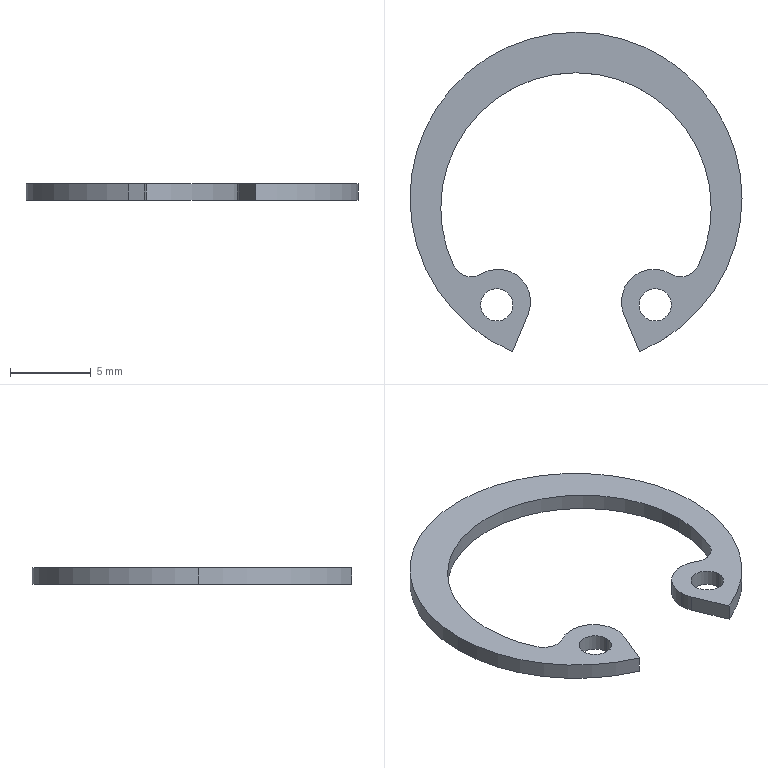Part | NX | features BREP 1 | 1 solid | 19 faces | box 20.5 x 19.72 x 1 mm | volume 114.602 mm3 | cylinder 15 | plane 4 | commonest cylinder face diameters 2 x4 4 x3 16.7 x3 20.5 x3 2.4 x2
STEP:
#1=CARTESIAN_POINT('',(-2.96,-7.147,-0.5));
#2=VERTEX_POINT('',#1);
#3=CARTESIAN_POINT('',(-5.846,-4.672,-0.5));
#4=VERTEX_POINT('',#3);
#5=CARTESIAN_POINT('',(-4.808,-6.381,-0.5));
#6=DIRECTION('',(0.,0.,1.));
#7=DIRECTION('',(1.,0.,0.));
#8=AXIS2_PLACEMENT_3D('',#5,#6,#7);
#9=CIRCLE('',#8,2.);
#10=EDGE_CURVE('',#2,#4,#9,.T.);
#11=ORIENTED_EDGE('',*,*,#10,.F.);
#12=CARTESIAN_POINT('',(-3.923,-9.47,-0.5));
#13=VERTEX_POINT('',#12);
#14=CARTESIAN_POINT('',(-2.96,-7.147,-0.5));
#15=DIRECTION('',(0.3827,0.9239,0.));
#16=VECTOR('',#15,1000.);
#17=LINE('',#14,#16);
#18=EDGE_CURVE('',#13,#2,#17,.T.);
#19=ORIENTED_EDGE('',*,*,#18,.F.);
#20=CARTESIAN_POINT('',(-10.25,0.,-0.5));
#21=VERTEX_POINT('',#20);
#22=CARTESIAN_POINT('',(0.,0.,-0.5));
#23=DIRECTION('',(0.,0.,1.));
#24=DIRECTION('',(1.,0.,0.));
#25=AXIS2_PLACEMENT_3D('',#22,#23,#24);
#26=CIRCLE('',#25,10.25);
#27=EDGE_CURVE('',#21,#13,#26,.T.);
#28=ORIENTED_EDGE('',*,*,#27,.F.);
#29=CARTESIAN_POINT('',(10.25,0.,-0.5));
#30=VERTEX_POINT('',#29);
#31=CARTESIAN_POINT('',(0.,0.,-0.5));
#32=DIRECTION('',(0.,0.,1.));
#33=DIRECTION('',(1.,0.,0.));
#34=AXIS2_PLACEMENT_3D('',#31,#32,#33);
#35=CIRCLE('',#34,10.25);
#36=EDGE_CURVE('',#30,#21,#35,.T.);
#37=ORIENTED_EDGE('',*,*,#36,.F.);
#38=CARTESIAN_POINT('',(3.923,-9.47,-0.5));
#39=VERTEX_POINT('',#38);
#40=CARTESIAN_POINT('',(0.,0.,-0.5));
#41=DIRECTION('',(0.,0.,1.));
#42=DIRECTION('',(1.,0.,0.));
#43=AXIS2_PLACEMENT_3D('',#40,#41,#42);
#44=CIRCLE('',#43,10.25);
#45=EDGE_CURVE('',#39,#30,#44,.T.);
#46=ORIENTED_EDGE('',*,*,#45,.F.);
#47=CARTESIAN_POINT('',(2.96,-7.147,-0.5));
#48=VERTEX_POINT('',#47);
#49=CARTESIAN_POINT('',(2.96,-7.147,-0.5));
#50=DIRECTION('',(0.3827,-0.9239,0.));
#51=VECTOR('',#50,1000.);
#52=LINE('',#49,#51);
#53=EDGE_CURVE('',#48,#39,#52,.T.);
#54=ORIENTED_EDGE('',*,*,#53,.F.);
#55=CARTESIAN_POINT('',(2.808,-6.381,-0.5));
#56=VERTEX_POINT('',#55);
#57=CARTESIAN_POINT('',(4.808,-6.381,-0.5));
#58=DIRECTION('',(0.,0.,1.));
#59=DIRECTION('',(-1.,0.,0.));
#60=AXIS2_PLACEMENT_3D('',#57,#58,#59);
#61=CIRCLE('',#60,2.);
#62=EDGE_CURVE('',#56,#48,#61,.T.);
#63=ORIENTED_EDGE('',*,*,#62,.F.);
#64=CARTESIAN_POINT('',(5.846,-4.672,-0.5));
#65=VERTEX_POINT('',#64);
#66=CARTESIAN_POINT('',(4.808,-6.381,-0.5));
#67=DIRECTION('',(0.,0.,1.));
#68=DIRECTION('',(-1.,0.,0.));
#69=AXIS2_PLACEMENT_3D('',#66,#67,#68);
#70=CIRCLE('',#69,2.);
#71=EDGE_CURVE('',#65,#56,#70,.T.);
#72=ORIENTED_EDGE('',*,*,#71,.F.);
#73=CARTESIAN_POINT('',(7.554,-4.157,-0.5));
#74=VERTEX_POINT('',#73);
#75=CARTESIAN_POINT('',(6.469,-3.646,-0.5));
#76=DIRECTION('',(0.,0.,-1.));
#77=DIRECTION('',(1.,0.,0.));
#78=AXIS2_PLACEMENT_3D('',#75,#76,#77);
#79=CIRCLE('',#78,1.2);
#80=EDGE_CURVE('',#74,#65,#79,.T.);
#81=ORIENTED_EDGE('',*,*,#80,.F.);
#82=CARTESIAN_POINT('',(8.35,-0.6,-0.5));
#83=VERTEX_POINT('',#82);
#84=CARTESIAN_POINT('',(0.,-0.6,-0.5));
#85=DIRECTION('',(0.,0.,-1.));
#86=DIRECTION('',(1.,0.,0.));
#87=AXIS2_PLACEMENT_3D('',#84,#85,#86);
#88=CIRCLE('',#87,8.35);
#89=EDGE_CURVE('',#83,#74,#88,.T.);
#90=ORIENTED_EDGE('',*,*,#89,.F.);
#91=CARTESIAN_POINT('',(-8.35,-0.6,-0.5));
#92=VERTEX_POINT('',#91);
#93=CARTESIAN_POINT('',(0.,-0.6,-0.5));
#94=DIRECTION('',(0.,0.,-1.));
#95=DIRECTION('',(1.,0.,0.));
#96=AXIS2_PLACEMENT_3D('',#93,#94,#95);
#97=CIRCLE('',#96,8.35);
#98=EDGE_CURVE('',#92,#83,#97,.T.);
#99=ORIENTED_EDGE('',*,*,#98,.F.);
#100=CARTESIAN_POINT('',(-7.554,-4.157,-0.5));
#101=VERTEX_POINT('',#100);
#102=CARTESIAN_POINT('',(0.,-0.6,-0.5));
#103=DIRECTION('',(0.,0.,-1.));
#104=DIRECTION('',(1.,0.,0.));
#105=AXIS2_PLACEMENT_3D('',#102,#103,#104);
#106=CIRCLE('',#105,8.35);
#107=EDGE_CURVE('',#101,#92,#106,.T.);
#108=ORIENTED_EDGE('',*,*,#107,.F.);
#109=CARTESIAN_POINT('',(-6.469,-3.646,-0.5));
#110=DIRECTION('',(0.,0.,-1.));
#111=DIRECTION('',(-1.,0.,0.));
#112=AXIS2_PLACEMENT_3D('',#109,#110,#111);
#113=CIRCLE('',#112,1.2);
#114=EDGE_CURVE('',#4,#101,#113,.T.);
#115=ORIENTED_EDGE('',*,*,#114,.F.);
#116=EDGE_LOOP('',(#11,#19,#28,#37,#46,#54,#63,#72,#81,#90,#99,#108,#115));
#117=FACE_BOUND('',#116,.T.);
#118=CARTESIAN_POINT('',(-5.891,-6.582,-0.5));
#119=VERTEX_POINT('',#118);
#120=CARTESIAN_POINT('',(-3.891,-6.582,-0.5));
#121=VERTEX_POINT('',#120);
#122=CARTESIAN_POINT('',(-4.891,-6.582,-0.5));
#123=DIRECTION('',(0.,0.,1.));
#124=DIRECTION('',(1.,0.,0.));
#125=AXIS2_PLACEMENT_3D('',#122,#123,#124);
#126=CIRCLE('',#125,1.);
#127=EDGE_CURVE('',#119,#121,#126,.T.);
#128=ORIENTED_EDGE('',*,*,#127,.T.);
#129=CARTESIAN_POINT('',(-4.891,-6.582,-0.5));
#130=DIRECTION('',(0.,0.,1.));
#131=DIRECTION('',(1.,0.,0.));
#132=AXIS2_PLACEMENT_3D('',#129,#130,#131);
#133=CIRCLE('',#132,1.);
#134=EDGE_CURVE('',#121,#119,#133,.T.);
#135=ORIENTED_EDGE('',*,*,#134,.T.);
#136=EDGE_LOOP('',(#128,#135));
#137=FACE_BOUND('',#136,.T.);
#138=CARTESIAN_POINT('',(3.891,-6.582,-0.5));
#139=VERTEX_POINT('',#138);
#140=CARTESIAN_POINT('',(5.891,-6.582,-0.5));
#141=VERTEX_POINT('',#140);
#142=CARTESIAN_POINT('',(4.891,-6.582,-0.5));
#143=DIRECTION('',(0.,0.,1.));
#144=DIRECTION('',(-1.,0.,0.));
#145=AXIS2_PLACEMENT_3D('',#142,#143,#144);
#146=CIRCLE('',#145,1.);
#147=EDGE_CURVE('',#139,#141,#146,.T.);
#148=ORIENTED_EDGE('',*,*,#147,.T.);
#149=CARTESIAN_POINT('',(4.891,-6.582,-0.5));
#150=DIRECTION('',(0.,0.,1.));
#151=DIRECTION('',(-1.,0.,0.));
#152=AXIS2_PLACEMENT_3D('',#149,#150,#151);
#153=CIRCLE('',#152,1.);
#154=EDGE_CURVE('',#141,#139,#153,.T.);
#155=ORIENTED_EDGE('',*,*,#154,.T.);
#156=EDGE_LOOP('',(#148,#155));
#157=FACE_BOUND('',#156,.T.);
#158=CARTESIAN_POINT('',(-4.808,-6.381,-0.5));
#159=DIRECTION('',(0.,0.,1.));
#160=DIRECTION('',(1.,0.,0.));
#161=AXIS2_PLACEMENT_3D('',#158,#159,#160);
#162=PLANE('',#161);
#163=ADVANCED_FACE('',(#117,#137,#157),#162,.F.);
#164=CARTESIAN_POINT('',(5.891,-6.582,0.5));
#165=VERTEX_POINT('',#164);
#166=CARTESIAN_POINT('',(5.891,-6.582,0.5));
#167=DIRECTION('',(0.,0.,-1.));
#168=VECTOR('',#167,1000.);
#169=LINE('',#166,#168);
#170=EDGE_CURVE('',#165,#141,#169,.T.);
#171=ORIENTED_EDGE('',*,*,#170,.F.);
#172=CARTESIAN_POINT('',(3.891,-6.582,0.5));
#173=VERTEX_POINT('',#172);
#174=CARTESIAN_POINT('',(4.891,-6.582,0.5));
#175=DIRECTION('',(0.,0.,1.));
#176=DIRECTION('',(-1.,0.,0.));
#177=AXIS2_PLACEMENT_3D('',#174,#175,#176);
#178=CIRCLE('',#177,1.);
#179=EDGE_CURVE('',#165,#173,#178,.T.);
#180=ORIENTED_EDGE('',*,*,#179,.T.);
#181=CARTESIAN_POINT('',(3.891,-6.582,0.5));
#182=DIRECTION('',(0.,0.,-1.));
#183=VECTOR('',#182,1000.);
#184=LINE('',#181,#183);
#185=EDGE_CURVE('',#173,#139,#184,.T.);
#186=ORIENTED_EDGE('',*,*,#185,.T.);
#187=ORIENTED_EDGE('',*,*,#154,.F.);
#188=EDGE_LOOP('',(#171,#180,#186,#187));
#189=FACE_BOUND('',#188,.T.);
#190=CARTESIAN_POINT('',(4.891,-6.582,0.5));
#191=DIRECTION('',(0.,0.,-1.));
#192=DIRECTION('',(-1.,0.,0.));
#193=AXIS2_PLACEMENT_3D('',#190,#191,#192);
#194=CYLINDRICAL_SURFACE('',#193,1.);
#195=ADVANCED_FACE('',(#189),#194,.F.);
#196=CARTESIAN_POINT('',(-3.891,-6.582,0.5));
#197=VERTEX_POINT('',#196);
#198=CARTESIAN_POINT('',(-3.891,-6.582,0.5));
#199=DIRECTION('',(0.,0.,-1.));
#200=VECTOR('',#199,1000.);
#201=LINE('',#198,#200);
#202=EDGE_CURVE('',#197,#121,#201,.T.);
#203=ORIENTED_EDGE('',*,*,#202,.F.);
#204=CARTESIAN_POINT('',(-5.891,-6.582,0.5));
#205=VERTEX_POINT('',#204);
#206=CARTESIAN_POINT('',(-4.891,-6.582,0.5));
#207=DIRECTION('',(0.,0.,1.));
#208=DIRECTION('',(1.,0.,0.));
#209=AXIS2_PLACEMENT_3D('',#206,#207,#208);
#210=CIRCLE('',#209,1.);
#211=EDGE_CURVE('',#197,#205,#210,.T.);
#212=ORIENTED_EDGE('',*,*,#211,.T.);
#213=CARTESIAN_POINT('',(-5.891,-6.582,0.5));
#214=DIRECTION('',(0.,0.,-1.));
#215=VECTOR('',#214,1000.);
#216=LINE('',#213,#215);
#217=EDGE_CURVE('',#205,#119,#216,.T.);
#218=ORIENTED_EDGE('',*,*,#217,.T.);
#219=ORIENTED_EDGE('',*,*,#134,.F.);
#220=EDGE_LOOP('',(#203,#212,#218,#219));
#221=FACE_BOUND('',#220,.T.);
#222=CARTESIAN_POINT('',(-4.891,-6.582,0.5));
#223=DIRECTION('',(0.,0.,-1.));
#224=DIRECTION('',(-1.,0.,0.));
#225=AXIS2_PLACEMENT_3D('',#222,#223,#224);
#226=CYLINDRICAL_SURFACE('',#225,1.);
#227=ADVANCED_FACE('',(#221),#226,.F.);
#228=CARTESIAN_POINT('',(-3.923,-9.47,0.5));
#229=VERTEX_POINT('',#228);
#230=CARTESIAN_POINT('',(-3.923,-9.47,0.5));
#231=DIRECTION('',(0.,0.,-1.));
#232=VECTOR('',#231,1000.);
#233=LINE('',#230,#232);
#234=EDGE_CURVE('',#229,#13,#233,.T.);
#235=ORIENTED_EDGE('',*,*,#234,.T.);
#236=ORIENTED_EDGE('',*,*,#18,.T.);
#237=CARTESIAN_POINT('',(-2.96,-7.147,0.5));
#238=VERTEX_POINT('',#237);
#239=CARTESIAN_POINT('',(-2.96,-7.147,0.5));
#240=DIRECTION('',(0.,0.,-1.));
#241=VECTOR('',#240,1000.);
#242=LINE('',#239,#241);
#243=EDGE_CURVE('',#238,#2,#242,.T.);
#244=ORIENTED_EDGE('',*,*,#243,.F.);
#245=CARTESIAN_POINT('',(-2.96,-7.147,0.5));
#246=DIRECTION('',(0.3827,0.9239,0.));
#247=VECTOR('',#246,1000.);
#248=LINE('',#245,#247);
#249=EDGE_CURVE('',#229,#238,#248,.T.);
#250=ORIENTED_EDGE('',*,*,#249,.F.);
#251=EDGE_LOOP('',(#235,#236,#244,#250));
#252=FACE_BOUND('',#251,.T.);
#253=CARTESIAN_POINT('',(-2.96,-7.147,0.5));
#254=DIRECTION('',(-0.9239,0.3827,0.));
#255=DIRECTION('',(-0.3827,-0.9239,0.));
#256=AXIS2_PLACEMENT_3D('',#253,#254,#255);
#257=PLANE('',#256);
#258=ADVANCED_FACE('',(#252),#257,.F.);
#259=CARTESIAN_POINT('',(10.25,0.,0.5));
#260=VERTEX_POINT('',#259);
#261=CARTESIAN_POINT('',(10.25,0.,0.5));
#262=DIRECTION('',(0.,0.,-1.));
#263=VECTOR('',#262,1000.);
#264=LINE('',#261,#263);
#265=EDGE_CURVE('',#260,#30,#264,.T.);
#266=ORIENTED_EDGE('',*,*,#265,.F.);
#267=CARTESIAN_POINT('',(3.923,-9.47,0.5));
#268=VERTEX_POINT('',#267);
#269=CARTESIAN_POINT('',(0.,0.,0.5));
#270=DIRECTION('',(0.,0.,1.));
#271=DIRECTION('',(1.,0.,0.));
#272=AXIS2_PLACEMENT_3D('',#269,#270,#271);
#273=CIRCLE('',#272,10.25);
#274=EDGE_CURVE('',#268,#260,#273,.T.);
#275=ORIENTED_EDGE('',*,*,#274,.F.);
#276=CARTESIAN_POINT('',(3.923,-9.47,0.5));
#277=DIRECTION('',(0.,0.,-1.));
#278=VECTOR('',#277,1000.);
#279=LINE('',#276,#278);
#280=EDGE_CURVE('',#268,#39,#279,.T.);
#281=ORIENTED_EDGE('',*,*,#280,.T.);
#282=ORIENTED_EDGE('',*,*,#45,.T.);
#283=EDGE_LOOP('',(#266,#275,#281,#282));
#284=FACE_BOUND('',#283,.T.);
#285=CARTESIAN_POINT('',(0.,0.,0.5));
#286=DIRECTION('',(0.,0.,-1.));
#287=DIRECTION('',(-1.,0.,0.));
#288=AXIS2_PLACEMENT_3D('',#285,#286,#287);
#289=CYLINDRICAL_SURFACE('',#288,10.25);
#290=ADVANCED_FACE('',(#284),#289,.T.);
#291=CARTESIAN_POINT('',(2.96,-7.147,0.5));
#292=VERTEX_POINT('',#291);
#293=CARTESIAN_POINT('',(2.96,-7.147,0.5));
#294=DIRECTION('',(0.,0.,-1.));
#295=VECTOR('',#294,1000.);
#296=LINE('',#293,#295);
#297=EDGE_CURVE('',#292,#48,#296,.T.);
#298=ORIENTED_EDGE('',*,*,#297,.T.);
#299=ORIENTED_EDGE('',*,*,#53,.T.);
#300=ORIENTED_EDGE('',*,*,#280,.F.);
#301=CARTESIAN_POINT('',(2.96,-7.147,0.5));
#302=DIRECTION('',(0.3827,-0.9239,0.));
#303=VECTOR('',#302,1000.);
#304=LINE('',#301,#303);
#305=EDGE_CURVE('',#292,#268,#304,.T.);
#306=ORIENTED_EDGE('',*,*,#305,.F.);
#307=EDGE_LOOP('',(#298,#299,#300,#306));
#308=FACE_BOUND('',#307,.T.);
#309=CARTESIAN_POINT('',(2.96,-7.147,0.5));
#310=DIRECTION('',(0.9239,0.3827,0.));
#311=DIRECTION('',(-0.3827,0.9239,0.));
#312=AXIS2_PLACEMENT_3D('',#309,#310,#311);
#313=PLANE('',#312);
#314=ADVANCED_FACE('',(#308),#313,.F.);
#315=CARTESIAN_POINT('',(2.808,-6.381,0.5));
#316=VERTEX_POINT('',#315);
#317=CARTESIAN_POINT('',(2.808,-6.381,0.5));
#318=DIRECTION('',(0.,0.,-1.));
#319=VECTOR('',#318,1000.);
#320=LINE('',#317,#319);
#321=EDGE_CURVE('',#316,#56,#320,.T.);
#322=ORIENTED_EDGE('',*,*,#321,.F.);
#323=CARTESIAN_POINT('',(5.846,-4.672,0.5));
#324=VERTEX_POINT('',#323);
#325=CARTESIAN_POINT('',(4.808,-6.381,0.5));
#326=DIRECTION('',(0.,0.,1.));
#327=DIRECTION('',(-1.,0.,0.));
#328=AXIS2_PLACEMENT_3D('',#325,#326,#327);
#329=CIRCLE('',#328,2.);
#330=EDGE_CURVE('',#324,#316,#329,.T.);
#331=ORIENTED_EDGE('',*,*,#330,.F.);
#332=CARTESIAN_POINT('',(5.846,-4.672,0.5));
#333=DIRECTION('',(0.,0.,-1.));
#334=VECTOR('',#333,1000.);
#335=LINE('',#332,#334);
#336=EDGE_CURVE('',#324,#65,#335,.T.);
#337=ORIENTED_EDGE('',*,*,#336,.T.);
#338=ORIENTED_EDGE('',*,*,#71,.T.);
#339=EDGE_LOOP('',(#322,#331,#337,#338));
#340=FACE_BOUND('',#339,.T.);
#341=CARTESIAN_POINT('',(4.808,-6.381,0.5));
#342=DIRECTION('',(0.,0.,-1.));
#343=DIRECTION('',(-1.,0.,0.));
#344=AXIS2_PLACEMENT_3D('',#341,#342,#343);
#345=CYLINDRICAL_SURFACE('',#344,2.);
#346=ADVANCED_FACE('',(#340),#345,.T.);
#347=CARTESIAN_POINT('',(7.554,-4.157,0.5));
#348=VERTEX_POINT('',#347);
#349=CARTESIAN_POINT('',(7.554,-4.157,0.5));
#350=DIRECTION('',(0.,0.,-1.));
#351=VECTOR('',#350,1000.);
#352=LINE('',#349,#351);
#353=EDGE_CURVE('',#348,#74,#352,.T.);
#354=ORIENTED_EDGE('',*,*,#353,.T.);
#355=ORIENTED_EDGE('',*,*,#80,.T.);
#356=ORIENTED_EDGE('',*,*,#336,.F.);
#357=CARTESIAN_POINT('',(6.469,-3.646,0.5));
#358=DIRECTION('',(0.,0.,-1.));
#359=DIRECTION('',(1.,0.,0.));
#360=AXIS2_PLACEMENT_3D('',#357,#358,#359);
#361=CIRCLE('',#360,1.2);
#362=EDGE_CURVE('',#348,#324,#361,.T.);
#363=ORIENTED_EDGE('',*,*,#362,.F.);
#364=EDGE_LOOP('',(#354,#355,#356,#363));
#365=FACE_BOUND('',#364,.T.);
#366=CARTESIAN_POINT('',(6.469,-3.646,0.5));
#367=DIRECTION('',(0.,0.,-1.));
#368=DIRECTION('',(-1.,0.,0.));
#369=AXIS2_PLACEMENT_3D('',#366,#367,#368);
#370=CYLINDRICAL_SURFACE('',#369,1.2);
#371=ADVANCED_FACE('',(#365),#370,.F.);
#372=CARTESIAN_POINT('',(-8.35,-0.6,0.5));
#373=VERTEX_POINT('',#372);
#374=CARTESIAN_POINT('',(-8.35,-0.6,0.5));
#375=DIRECTION('',(0.,0.,-1.));
#376=VECTOR('',#375,1000.);
#377=LINE('',#374,#376);
#378=EDGE_CURVE('',#373,#92,#377,.T.);
#379=ORIENTED_EDGE('',*,*,#378,.F.);
#380=CARTESIAN_POINT('',(-7.554,-4.157,0.5));
#381=VERTEX_POINT('',#380);
#382=CARTESIAN_POINT('',(0.,-0.6,0.5));
#383=DIRECTION('',(0.,0.,-1.));
#384=DIRECTION('',(1.,0.,0.));
#385=AXIS2_PLACEMENT_3D('',#382,#383,#384);
#386=CIRCLE('',#385,8.35);
#387=EDGE_CURVE('',#381,#373,#386,.T.);
#388=ORIENTED_EDGE('',*,*,#387,.F.);
#389=CARTESIAN_POINT('',(-7.554,-4.157,0.5));
#390=DIRECTION('',(0.,0.,-1.));
#391=VECTOR('',#390,1000.);
#392=LINE('',#389,#391);
#393=EDGE_CURVE('',#381,#101,#392,.T.);
#394=ORIENTED_EDGE('',*,*,#393,.T.);
#395=ORIENTED_EDGE('',*,*,#107,.T.);
#396=EDGE_LOOP('',(#379,#388,#394,#395));
#397=FACE_BOUND('',#396,.T.);
#398=CARTESIAN_POINT('',(0.,-0.6,0.5));
#399=DIRECTION('',(0.,0.,-1.));
#400=DIRECTION('',(-1.,0.,0.));
#401=AXIS2_PLACEMENT_3D('',#398,#399,#400);
#402=CYLINDRICAL_SURFACE('',#401,8.35);
#403=ADVANCED_FACE('',(#397),#402,.F.);
#404=CARTESIAN_POINT('',(-5.846,-4.672,0.5));
#405=VERTEX_POINT('',#404);
#406=CARTESIAN_POINT('',(-5.846,-4.672,0.5));
#407=DIRECTION('',(0.,0.,-1.));
#408=VECTOR('',#407,1000.);
#409=LINE('',#406,#408);
#410=EDGE_CURVE('',#405,#4,#409,.T.);
#411=ORIENTED_EDGE('',*,*,#410,.T.);
#412=ORIENTED_EDGE('',*,*,#114,.T.);
#413=ORIENTED_EDGE('',*,*,#393,.F.);
#414=CARTESIAN_POINT('',(-6.469,-3.646,0.5));
#415=DIRECTION('',(0.,0.,-1.));
#416=DIRECTION('',(-1.,0.,0.));
#417=AXIS2_PLACEMENT_3D('',#414,#415,#416);
#418=CIRCLE('',#417,1.2);
#419=EDGE_CURVE('',#405,#381,#418,.T.);
#420=ORIENTED_EDGE('',*,*,#419,.F.);
#421=EDGE_LOOP('',(#411,#412,#413,#420));
#422=FACE_BOUND('',#421,.T.);
#423=CARTESIAN_POINT('',(-6.469,-3.646,0.5));
#424=DIRECTION('',(0.,0.,-1.));
#425=DIRECTION('',(-1.,0.,0.));
#426=AXIS2_PLACEMENT_3D('',#423,#424,#425);
#427=CYLINDRICAL_SURFACE('',#426,1.2);
#428=ADVANCED_FACE('',(#422),#427,.F.);
#429=ORIENTED_EDGE('',*,*,#243,.T.);
#430=ORIENTED_EDGE('',*,*,#10,.T.);
#431=ORIENTED_EDGE('',*,*,#410,.F.);
#432=CARTESIAN_POINT('',(-4.808,-6.381,0.5));
#433=DIRECTION('',(0.,0.,1.));
#434=DIRECTION('',(1.,0.,0.));
#435=AXIS2_PLACEMENT_3D('',#432,#433,#434);
#436=CIRCLE('',#435,2.);
#437=EDGE_CURVE('',#238,#405,#436,.T.);
#438=ORIENTED_EDGE('',*,*,#437,.F.);
#439=EDGE_LOOP('',(#429,#430,#431,#438));
#440=FACE_BOUND('',#439,.T.);
#441=CARTESIAN_POINT('',(-4.808,-6.381,0.5));
#442=DIRECTION('',(0.,0.,-1.));
#443=DIRECTION('',(-1.,0.,0.));
#444=AXIS2_PLACEMENT_3D('',#441,#442,#443);
#445=CYLINDRICAL_SURFACE('',#444,2.);
#446=ADVANCED_FACE('',(#440),#445,.T.);
#447=CARTESIAN_POINT('',(4.891,-6.582,0.5));
#448=DIRECTION('',(0.,0.,1.));
#449=DIRECTION('',(-1.,0.,0.));
#450=AXIS2_PLACEMENT_3D('',#447,#448,#449);
#451=CIRCLE('',#450,1.);
#452=EDGE_CURVE('',#173,#165,#451,.T.);
#453=ORIENTED_EDGE('',*,*,#452,.F.);
#454=ORIENTED_EDGE('',*,*,#179,.F.);
#455=EDGE_LOOP('',(#453,#454));
#456=FACE_BOUND('',#455,.T.);
#457=ORIENTED_EDGE('',*,*,#437,.T.);
#458=ORIENTED_EDGE('',*,*,#419,.T.);
#459=ORIENTED_EDGE('',*,*,#387,.T.);
#460=CARTESIAN_POINT('',(8.35,-0.6,0.5));
#461=VERTEX_POINT('',#460);
#462=CARTESIAN_POINT('',(0.,-0.6,0.5));
#463=DIRECTION('',(0.,0.,-1.));
#464=DIRECTION('',(1.,0.,0.));
#465=AXIS2_PLACEMENT_3D('',#462,#463,#464);
#466=CIRCLE('',#465,8.35);
#467=EDGE_CURVE('',#373,#461,#466,.T.);
#468=ORIENTED_EDGE('',*,*,#467,.T.);
#469=CARTESIAN_POINT('',(0.,-0.6,0.5));
#470=DIRECTION('',(0.,0.,-1.));
#471=DIRECTION('',(1.,0.,0.));
#472=AXIS2_PLACEMENT_3D('',#469,#470,#471);
#473=CIRCLE('',#472,8.35);
#474=EDGE_CURVE('',#461,#348,#473,.T.);
#475=ORIENTED_EDGE('',*,*,#474,.T.);
#476=ORIENTED_EDGE('',*,*,#362,.T.);
#477=ORIENTED_EDGE('',*,*,#330,.T.);
#478=CARTESIAN_POINT('',(4.808,-6.381,0.5));
#479=DIRECTION('',(0.,0.,1.));
#480=DIRECTION('',(-1.,0.,0.));
#481=AXIS2_PLACEMENT_3D('',#478,#479,#480);
#482=CIRCLE('',#481,2.);
#483=EDGE_CURVE('',#316,#292,#482,.T.);
#484=ORIENTED_EDGE('',*,*,#483,.T.);
#485=ORIENTED_EDGE('',*,*,#305,.T.);
#486=ORIENTED_EDGE('',*,*,#274,.T.);
#487=CARTESIAN_POINT('',(-10.25,0.,0.5));
#488=VERTEX_POINT('',#487);
#489=CARTESIAN_POINT('',(0.,0.,0.5));
#490=DIRECTION('',(0.,0.,1.));
#491=DIRECTION('',(1.,0.,0.));
#492=AXIS2_PLACEMENT_3D('',#489,#490,#491);
#493=CIRCLE('',#492,10.25);
#494=EDGE_CURVE('',#260,#488,#493,.T.);
#495=ORIENTED_EDGE('',*,*,#494,.T.);
#496=CARTESIAN_POINT('',(0.,0.,0.5));
#497=DIRECTION('',(0.,0.,1.));
#498=DIRECTION('',(1.,0.,0.));
#499=AXIS2_PLACEMENT_3D('',#496,#497,#498);
#500=CIRCLE('',#499,10.25);
#501=EDGE_CURVE('',#488,#229,#500,.T.);
#502=ORIENTED_EDGE('',*,*,#501,.T.);
#503=ORIENTED_EDGE('',*,*,#249,.T.);
#504=EDGE_LOOP('',(#457,#458,#459,#468,#475,#476,#477,#484,#485,#486,#495,#502,#503));
#505=FACE_BOUND('',#504,.T.);
#506=CARTESIAN_POINT('',(-4.891,-6.582,0.5));
#507=DIRECTION('',(0.,0.,1.));
#508=DIRECTION('',(1.,0.,0.));
#509=AXIS2_PLACEMENT_3D('',#506,#507,#508);
#510=CIRCLE('',#509,1.);
#511=EDGE_CURVE('',#205,#197,#510,.T.);
#512=ORIENTED_EDGE('',*,*,#511,.F.);
#513=ORIENTED_EDGE('',*,*,#211,.F.);
#514=EDGE_LOOP('',(#512,#513));
#515=FACE_BOUND('',#514,.T.);
#516=CARTESIAN_POINT('',(-4.808,-6.381,0.5));
#517=DIRECTION('',(0.,0.,1.));
#518=DIRECTION('',(1.,0.,0.));
#519=AXIS2_PLACEMENT_3D('',#516,#517,#518);
#520=PLANE('',#519);
#521=ADVANCED_FACE('',(#456,#505,#515),#520,.T.);
#522=CARTESIAN_POINT('',(8.35,-0.6,0.5));
#523=DIRECTION('',(0.,0.,-1.));
#524=VECTOR('',#523,1000.);
#525=LINE('',#522,#524);
#526=EDGE_CURVE('',#461,#83,#525,.T.);
#527=ORIENTED_EDGE('',*,*,#526,.F.);
#528=ORIENTED_EDGE('',*,*,#467,.F.);
#529=ORIENTED_EDGE('',*,*,#378,.T.);
#530=ORIENTED_EDGE('',*,*,#98,.T.);
#531=EDGE_LOOP('',(#527,#528,#529,#530));
#532=FACE_BOUND('',#531,.T.);
#533=CARTESIAN_POINT('',(0.,-0.6,0.5));
#534=DIRECTION('',(0.,0.,-1.));
#535=DIRECTION('',(-1.,0.,0.));
#536=AXIS2_PLACEMENT_3D('',#533,#534,#535);
#537=CYLINDRICAL_SURFACE('',#536,8.35);
#538=ADVANCED_FACE('',(#532),#537,.F.);
#539=ORIENTED_EDGE('',*,*,#474,.F.);
#540=ORIENTED_EDGE('',*,*,#526,.T.);
#541=ORIENTED_EDGE('',*,*,#89,.T.);
#542=ORIENTED_EDGE('',*,*,#353,.F.);
#543=EDGE_LOOP('',(#539,#540,#541,#542));
#544=FACE_BOUND('',#543,.T.);
#545=CARTESIAN_POINT('',(0.,-0.6,0.5));
#546=DIRECTION('',(0.,0.,-1.));
#547=DIRECTION('',(-1.,0.,0.));
#548=AXIS2_PLACEMENT_3D('',#545,#546,#547);
#549=CYLINDRICAL_SURFACE('',#548,8.35);
#550=ADVANCED_FACE('',(#544),#549,.F.);
#551=ORIENTED_EDGE('',*,*,#483,.F.);
#552=ORIENTED_EDGE('',*,*,#321,.T.);
#553=ORIENTED_EDGE('',*,*,#62,.T.);
#554=ORIENTED_EDGE('',*,*,#297,.F.);
#555=EDGE_LOOP('',(#551,#552,#553,#554));
#556=FACE_BOUND('',#555,.T.);
#557=CARTESIAN_POINT('',(4.808,-6.381,0.5));
#558=DIRECTION('',(0.,0.,-1.));
#559=DIRECTION('',(-1.,0.,0.));
#560=AXIS2_PLACEMENT_3D('',#557,#558,#559);
#561=CYLINDRICAL_SURFACE('',#560,2.);
#562=ADVANCED_FACE('',(#556),#561,.T.);
#563=ORIENTED_EDGE('',*,*,#501,.F.);
#564=CARTESIAN_POINT('',(-10.25,0.,0.5));
#565=DIRECTION('',(0.,0.,-1.));
#566=VECTOR('',#565,1000.);
#567=LINE('',#564,#566);
#568=EDGE_CURVE('',#488,#21,#567,.T.);
#569=ORIENTED_EDGE('',*,*,#568,.T.);
#570=ORIENTED_EDGE('',*,*,#27,.T.);
#571=ORIENTED_EDGE('',*,*,#234,.F.);
#572=EDGE_LOOP('',(#563,#569,#570,#571));
#573=FACE_BOUND('',#572,.T.);
#574=CARTESIAN_POINT('',(0.,0.,0.5));
#575=DIRECTION('',(0.,0.,-1.));
#576=DIRECTION('',(-1.,0.,0.));
#577=AXIS2_PLACEMENT_3D('',#574,#575,#576);
#578=CYLINDRICAL_SURFACE('',#577,10.25);
#579=ADVANCED_FACE('',(#573),#578,.T.);
#580=ORIENTED_EDGE('',*,*,#494,.F.);
#581=ORIENTED_EDGE('',*,*,#265,.T.);
#582=ORIENTED_EDGE('',*,*,#36,.T.);
#583=ORIENTED_EDGE('',*,*,#568,.F.);
#584=EDGE_LOOP('',(#580,#581,#582,#583));
#585=FACE_BOUND('',#584,.T.);
#586=CARTESIAN_POINT('',(0.,0.,0.5));
#587=DIRECTION('',(0.,0.,-1.));
#588=DIRECTION('',(-1.,0.,0.));
#589=AXIS2_PLACEMENT_3D('',#586,#587,#588);
#590=CYLINDRICAL_SURFACE('',#589,10.25);
#591=ADVANCED_FACE('',(#585),#590,.T.);
#592=ORIENTED_EDGE('',*,*,#511,.T.);
#593=ORIENTED_EDGE('',*,*,#202,.T.);
#594=ORIENTED_EDGE('',*,*,#127,.F.);
#595=ORIENTED_EDGE('',*,*,#217,.F.);
#596=EDGE_LOOP('',(#592,#593,#594,#595));
#597=FACE_BOUND('',#596,.T.);
#598=CARTESIAN_POINT('',(-4.891,-6.582,0.5));
#599=DIRECTION('',(0.,0.,-1.));
#600=DIRECTION('',(-1.,0.,0.));
#601=AXIS2_PLACEMENT_3D('',#598,#599,#600);
#602=CYLINDRICAL_SURFACE('',#601,1.);
#603=ADVANCED_FACE('',(#597),#602,.F.);
#604=ORIENTED_EDGE('',*,*,#452,.T.);
#605=ORIENTED_EDGE('',*,*,#170,.T.);
#606=ORIENTED_EDGE('',*,*,#147,.F.);
#607=ORIENTED_EDGE('',*,*,#185,.F.);
#608=EDGE_LOOP('',(#604,#605,#606,#607));
#609=FACE_BOUND('',#608,.T.);
#610=CARTESIAN_POINT('',(4.891,-6.582,0.5));
#611=DIRECTION('',(0.,0.,-1.));
#612=DIRECTION('',(-1.,0.,0.));
#613=AXIS2_PLACEMENT_3D('',#610,#611,#612);
#614=CYLINDRICAL_SURFACE('',#613,1.);
#615=ADVANCED_FACE('',(#609),#614,.F.);
#616=CLOSED_SHELL('',(#163,#195,#227,#258,#290,#314,#346,#371,#403,#428,#446,#521,#538,#550,#562,#579,#591,#603,#615));
#617=MANIFOLD_SOLID_BREP('',#616);
#618=(LENGTH_UNIT()NAMED_UNIT(*)SI_UNIT(.MILLI.,.METRE.));
#619=UNCERTAINTY_MEASURE_WITH_UNIT(LENGTH_MEASURE(0.00001),#618,'','');
#620=(NAMED_UNIT(*)PLANE_ANGLE_UNIT()SI_UNIT($,.RADIAN.));
#621=(NAMED_UNIT(*)SI_UNIT($,.STERADIAN.)SOLID_ANGLE_UNIT());
#622=(GEOMETRIC_REPRESENTATION_CONTEXT(3)GLOBAL_UNCERTAINTY_ASSIGNED_CONTEXT((#619))GLOBAL_UNIT_ASSIGNED_CONTEXT((#618,#620,#621))REPRESENTATION_CONTEXT('',''));
#623=ADVANCED_BREP_SHAPE_REPRESENTATION('',(#617),#622);